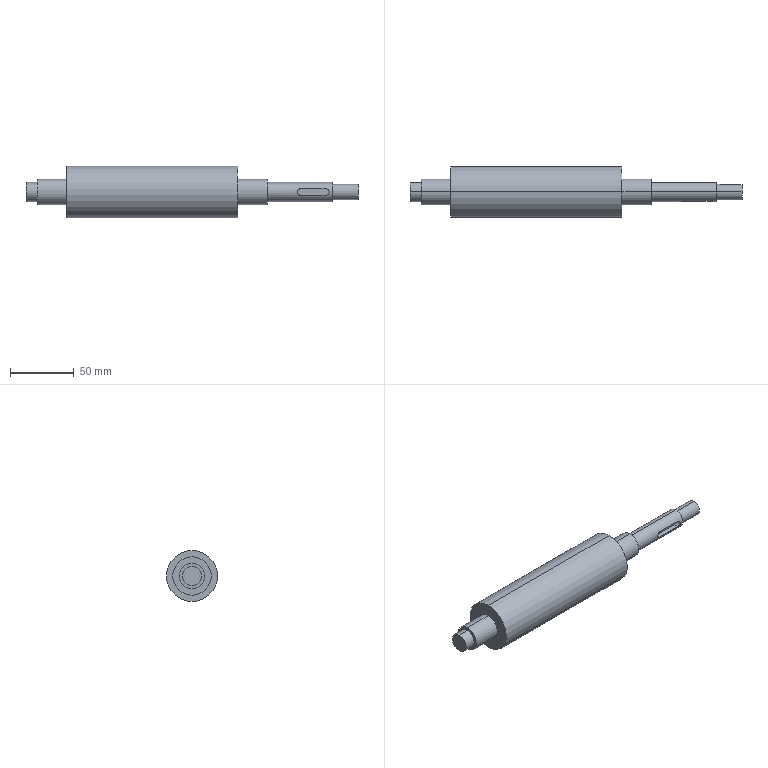Part | STEP file | MT-COMBO-119-S017 | 2 solids | 34 faces | box 260 x 40 x 40 mm | volume 195020 mm3 | cylinder 19 | plane 15 | commonest cylinder face diameters 15 x4 20 x4 30 x4 5 x2 12 x2 40 x2
STEP:
#1=CARTESIAN_POINT('',(-14.5,0.,-15.));
#2=VERTEX_POINT('',#1);
#3=CARTESIAN_POINT('',(-14.5,0.,15.));
#4=VERTEX_POINT('',#3);
#5=CARTESIAN_POINT('',(-14.5,0.,0.));
#6=DIRECTION('',(1.,0.,0.));
#7=DIRECTION('',(0.,0.,1.));
#8=AXIS2_PLACEMENT_3D('',#5,#6,#7);
#9=CIRCLE('',#8,15.);
#10=EDGE_CURVE('',#2,#4,#9,.T.);
#11=ORIENTED_EDGE('',*,*,#10,.F.);
#12=CARTESIAN_POINT('',(119.5,0.,-15.));
#13=VERTEX_POINT('',#12);
#14=CARTESIAN_POINT('',(-131.5,0.,-15.));
#15=DIRECTION('',(1.,0.,0.));
#16=VECTOR('',#15,1000.);
#17=LINE('',#14,#16);
#18=EDGE_CURVE('',#2,#13,#17,.T.);
#19=ORIENTED_EDGE('',*,*,#18,.T.);
#20=CARTESIAN_POINT('',(119.5,0.,15.));
#21=VERTEX_POINT('',#20);
#22=CARTESIAN_POINT('',(119.5,0.,0.));
#23=DIRECTION('',(-1.,0.,0.));
#24=DIRECTION('',(0.,0.,-1.));
#25=AXIS2_PLACEMENT_3D('',#22,#23,#24);
#26=CIRCLE('',#25,15.);
#27=EDGE_CURVE('',#21,#13,#26,.T.);
#28=ORIENTED_EDGE('',*,*,#27,.F.);
#29=CARTESIAN_POINT('',(-131.5,0.,15.));
#30=DIRECTION('',(1.,0.,0.));
#31=VECTOR('',#30,1000.);
#32=LINE('',#29,#31);
#33=EDGE_CURVE('',#4,#21,#32,.T.);
#34=ORIENTED_EDGE('',*,*,#33,.F.);
#35=EDGE_LOOP('',(#11,#19,#28,#34));
#36=FACE_OUTER_BOUND('',#35,.T.);
#37=CARTESIAN_POINT('',(-131.5,0.,0.));
#38=DIRECTION('',(1.,0.,0.));
#39=DIRECTION('',(0.,0.,1.));
#40=AXIS2_PLACEMENT_3D('',#37,#38,#39);
#41=CYLINDRICAL_SURFACE('',#40,15.);
#42=ADVANCED_FACE('',(#36),#41,.F.);
#43=CARTESIAN_POINT('',(-14.5,0.,-20.));
#44=VERTEX_POINT('',#43);
#45=CARTESIAN_POINT('',(-14.5,0.,20.));
#46=VERTEX_POINT('',#45);
#47=CARTESIAN_POINT('',(-14.5,0.,0.));
#48=DIRECTION('',(-1.,0.,0.));
#49=DIRECTION('',(0.,0.,1.));
#50=AXIS2_PLACEMENT_3D('',#47,#48,#49);
#51=CIRCLE('',#50,20.);
#52=EDGE_CURVE('',#44,#46,#51,.T.);
#53=ORIENTED_EDGE('',*,*,#52,.F.);
#54=CARTESIAN_POINT('',(119.5,0.,-20.));
#55=VERTEX_POINT('',#54);
#56=CARTESIAN_POINT('',(-131.5,0.,-20.));
#57=DIRECTION('',(1.,0.,0.));
#58=VECTOR('',#57,1000.);
#59=LINE('',#56,#58);
#60=EDGE_CURVE('',#44,#55,#59,.T.);
#61=ORIENTED_EDGE('',*,*,#60,.T.);
#62=CARTESIAN_POINT('',(119.5,0.,20.));
#63=VERTEX_POINT('',#62);
#64=CARTESIAN_POINT('',(119.5,0.,0.));
#65=DIRECTION('',(1.,0.,0.));
#66=DIRECTION('',(0.,0.,-1.));
#67=AXIS2_PLACEMENT_3D('',#64,#65,#66);
#68=CIRCLE('',#67,20.);
#69=EDGE_CURVE('',#63,#55,#68,.T.);
#70=ORIENTED_EDGE('',*,*,#69,.F.);
#71=CARTESIAN_POINT('',(-131.5,0.,20.));
#72=DIRECTION('',(1.,0.,0.));
#73=VECTOR('',#72,1000.);
#74=LINE('',#71,#73);
#75=EDGE_CURVE('',#46,#63,#74,.T.);
#76=ORIENTED_EDGE('',*,*,#75,.F.);
#77=EDGE_LOOP('',(#53,#61,#70,#76));
#78=FACE_OUTER_BOUND('',#77,.T.);
#79=CARTESIAN_POINT('',(-131.5,0.,0.));
#80=DIRECTION('',(1.,0.,0.));
#81=DIRECTION('',(0.,0.,1.));
#82=AXIS2_PLACEMENT_3D('',#79,#80,#81);
#83=CYLINDRICAL_SURFACE('',#82,20.);
#84=ADVANCED_FACE('',(#78),#83,.T.);
#85=ORIENTED_EDGE('',*,*,#60,.F.);
#86=CARTESIAN_POINT('',(-14.5,0.,0.));
#87=DIRECTION('',(-1.,0.,0.));
#88=DIRECTION('',(0.,0.,1.));
#89=AXIS2_PLACEMENT_3D('',#86,#87,#88);
#90=CIRCLE('',#89,20.);
#91=EDGE_CURVE('',#46,#44,#90,.T.);
#92=ORIENTED_EDGE('',*,*,#91,.F.);
#93=ORIENTED_EDGE('',*,*,#75,.T.);
#94=CARTESIAN_POINT('',(119.5,0.,0.));
#95=DIRECTION('',(1.,0.,0.));
#96=DIRECTION('',(0.,0.,-1.));
#97=AXIS2_PLACEMENT_3D('',#94,#95,#96);
#98=CIRCLE('',#97,20.);
#99=EDGE_CURVE('',#55,#63,#98,.T.);
#100=ORIENTED_EDGE('',*,*,#99,.F.);
#101=EDGE_LOOP('',(#85,#92,#93,#100));
#102=FACE_OUTER_BOUND('',#101,.T.);
#103=CARTESIAN_POINT('',(-131.5,0.,0.));
#104=DIRECTION('',(1.,0.,0.));
#105=DIRECTION('',(0.,0.,1.));
#106=AXIS2_PLACEMENT_3D('',#103,#104,#105);
#107=CYLINDRICAL_SURFACE('',#106,20.);
#108=ADVANCED_FACE('',(#102),#107,.T.);
#109=ORIENTED_EDGE('',*,*,#18,.F.);
#110=CARTESIAN_POINT('',(-14.5,0.,0.));
#111=DIRECTION('',(1.,0.,0.));
#112=DIRECTION('',(0.,0.,1.));
#113=AXIS2_PLACEMENT_3D('',#110,#111,#112);
#114=CIRCLE('',#113,15.);
#115=EDGE_CURVE('',#4,#2,#114,.T.);
#116=ORIENTED_EDGE('',*,*,#115,.F.);
#117=ORIENTED_EDGE('',*,*,#33,.T.);
#118=CARTESIAN_POINT('',(119.5,0.,0.));
#119=DIRECTION('',(-1.,0.,0.));
#120=DIRECTION('',(0.,0.,-1.));
#121=AXIS2_PLACEMENT_3D('',#118,#119,#120);
#122=CIRCLE('',#121,15.);
#123=EDGE_CURVE('',#13,#21,#122,.T.);
#124=ORIENTED_EDGE('',*,*,#123,.F.);
#125=EDGE_LOOP('',(#109,#116,#117,#124));
#126=FACE_OUTER_BOUND('',#125,.T.);
#127=CARTESIAN_POINT('',(-131.5,0.,0.));
#128=DIRECTION('',(1.,0.,0.));
#129=DIRECTION('',(0.,0.,1.));
#130=AXIS2_PLACEMENT_3D('',#127,#128,#129);
#131=CYLINDRICAL_SURFACE('',#130,15.);
#132=ADVANCED_FACE('',(#126),#131,.F.);
#133=ORIENTED_EDGE('',*,*,#91,.T.);
#134=ORIENTED_EDGE('',*,*,#52,.T.);
#135=EDGE_LOOP('',(#133,#134));
#136=FACE_OUTER_BOUND('',#135,.T.);
#137=ORIENTED_EDGE('',*,*,#115,.T.);
#138=ORIENTED_EDGE('',*,*,#10,.T.);
#139=EDGE_LOOP('',(#137,#138));
#140=FACE_BOUND('',#139,.T.);
#141=CARTESIAN_POINT('',(-14.5,0.,0.));
#142=DIRECTION('',(-1.,0.,0.));
#143=DIRECTION('',(0.,0.,1.));
#144=AXIS2_PLACEMENT_3D('',#141,#142,#143);
#145=PLANE('',#144);
#146=ADVANCED_FACE('',(#136,#140),#145,.T.);
#147=ORIENTED_EDGE('',*,*,#69,.T.);
#148=ORIENTED_EDGE('',*,*,#99,.T.);
#149=EDGE_LOOP('',(#147,#148));
#150=FACE_OUTER_BOUND('',#149,.T.);
#151=ORIENTED_EDGE('',*,*,#27,.T.);
#152=ORIENTED_EDGE('',*,*,#123,.T.);
#153=EDGE_LOOP('',(#151,#152));
#154=FACE_BOUND('',#153,.T.);
#155=CARTESIAN_POINT('',(119.5,0.,0.));
#156=DIRECTION('',(1.,0.,0.));
#157=DIRECTION('',(0.,0.,-1.));
#158=AXIS2_PLACEMENT_3D('',#155,#156,#157);
#159=PLANE('',#158);
#160=ADVANCED_FACE('',(#150,#154),#159,.T.);
#161=CLOSED_SHELL('',(#42,#84,#108,#132,#146,#160));
#162=MANIFOLD_SOLID_BREP('',#161);
#163=CARTESIAN_POINT('',(193.5,0.,-6.));
#164=VERTEX_POINT('',#163);
#165=CARTESIAN_POINT('',(193.5,0.,6.));
#166=VERTEX_POINT('',#165);
#167=CARTESIAN_POINT('',(193.5,0.,0.));
#168=DIRECTION('',(1.,0.,0.));
#169=DIRECTION('',(0.,0.,-1.));
#170=AXIS2_PLACEMENT_3D('',#167,#168,#169);
#171=CIRCLE('',#170,6.);
#172=EDGE_CURVE('',#164,#166,#171,.T.);
#173=ORIENTED_EDGE('',*,*,#172,.T.);
#174=CARTESIAN_POINT('',(213.5,0.,6.));
#175=VERTEX_POINT('',#174);
#176=CARTESIAN_POINT('',(193.5,0.,6.));
#177=DIRECTION('',(1.,0.,0.));
#178=VECTOR('',#177,1000.);
#179=LINE('',#176,#178);
#180=EDGE_CURVE('',#166,#175,#179,.T.);
#181=ORIENTED_EDGE('',*,*,#180,.T.);
#182=CARTESIAN_POINT('',(213.5,5.657,2.));
#183=VERTEX_POINT('',#182);
#184=CARTESIAN_POINT('',(213.5,0.,0.));
#185=DIRECTION('',(1.,0.,0.));
#186=DIRECTION('',(0.,0.,-1.));
#187=AXIS2_PLACEMENT_3D('',#184,#185,#186);
#188=CIRCLE('',#187,6.);
#189=EDGE_CURVE('',#183,#175,#188,.T.);
#190=ORIENTED_EDGE('',*,*,#189,.F.);
#191=CARTESIAN_POINT('',(198.,5.657,2.));
#192=VERTEX_POINT('',#191);
#193=CARTESIAN_POINT('',(193.5,5.657,2.));
#194=DIRECTION('',(1.,0.,0.));
#195=VECTOR('',#194,1000.);
#196=LINE('',#193,#195);
#197=EDGE_CURVE('',#192,#183,#196,.T.);
#198=ORIENTED_EDGE('',*,*,#197,.F.);
#199=CARTESIAN_POINT('',(198.,5.657,-2.));
#200=VERTEX_POINT('',#199);
#201=CARTESIAN_POINT('',(198.,5.657,-2.));
#202=CARTESIAN_POINT('',(197.867,5.657,-2.));
#203=CARTESIAN_POINT('',(197.736,5.662,-1.987));
#204=CARTESIAN_POINT('',(197.479,5.679,-1.935));
#205=CARTESIAN_POINT('',(197.352,5.693,-1.897));
#206=CARTESIAN_POINT('',(197.11,5.725,-1.796));
#207=CARTESIAN_POINT('',(196.996,5.744,-1.735));
#208=CARTESIAN_POINT('',(196.779,5.786,-1.59));
#209=CARTESIAN_POINT('',(196.677,5.809,-1.506));
#210=CARTESIAN_POINT('',(196.403,5.875,-1.231));
#211=CARTESIAN_POINT('',(196.254,5.919,-1.01));
#212=CARTESIAN_POINT('',(196.104,5.966,-0.6496));
#213=CARTESIAN_POINT('',(196.065,5.979,-0.5226));
#214=CARTESIAN_POINT('',(196.013,5.996,-0.264));
#215=CARTESIAN_POINT('',(196.,6.,-0.1336));
#216=CARTESIAN_POINT('',(196.,6.,0.1294));
#217=CARTESIAN_POINT('',(196.013,5.996,0.2629));
#218=CARTESIAN_POINT('',(196.064,5.979,0.5202));
#219=CARTESIAN_POINT('',(196.102,5.966,0.6454));
#220=CARTESIAN_POINT('',(196.204,5.935,0.8889));
#221=CARTESIAN_POINT('',(196.266,5.916,1.004));
#222=CARTESIAN_POINT('',(196.41,5.876,1.22));
#223=CARTESIAN_POINT('',(196.493,5.853,1.322));
#224=CARTESIAN_POINT('',(196.677,5.809,1.506));
#225=CARTESIAN_POINT('',(196.777,5.787,1.588));
#226=CARTESIAN_POINT('',(196.993,5.745,1.733));
#227=CARTESIAN_POINT('',(197.11,5.725,1.796));
#228=CARTESIAN_POINT('',(197.471,5.677,1.946));
#229=CARTESIAN_POINT('',(197.734,5.657,2.));
#230=CARTESIAN_POINT('',(198.,5.657,2.));
#231=B_SPLINE_CURVE_WITH_KNOTS('',3,(#201,#202,#203,#204,#205,#206,#207,#208,#209,#210,#211,#212,#213,#214,#215,#216,#217,#218,#219,#220,#221,#222,#223,#224,#225,#226,#227,#228,#229,#230),.UNSPECIFIED.,.F.,.F.,(4,2,2,2,2,2,2,2,2,2,2,2,2,2,4),(0.,0.0003935,0.000787,0.00118,0.001574,0.002361,0.002754,0.003148,0.003541,0.003935,0.004328,0.004722,0.005115,0.005509,0.006296),.UNSPECIFIED.);
#232=EDGE_CURVE('',#200,#192,#231,.T.);
#233=ORIENTED_EDGE('',*,*,#232,.F.);
#234=CARTESIAN_POINT('',(213.5,5.657,-2.));
#235=VERTEX_POINT('',#234);
#236=CARTESIAN_POINT('',(193.5,5.657,-2.));
#237=DIRECTION('',(-1.,0.,0.));
#238=VECTOR('',#237,1000.);
#239=LINE('',#236,#238);
#240=EDGE_CURVE('',#235,#200,#239,.T.);
#241=ORIENTED_EDGE('',*,*,#240,.F.);
#242=CARTESIAN_POINT('',(213.5,0.,-6.));
#243=VERTEX_POINT('',#242);
#244=CARTESIAN_POINT('',(213.5,0.,0.));
#245=DIRECTION('',(1.,0.,0.));
#246=DIRECTION('',(0.,0.,-1.));
#247=AXIS2_PLACEMENT_3D('',#244,#245,#246);
#248=CIRCLE('',#247,6.);
#249=EDGE_CURVE('',#243,#235,#248,.T.);
#250=ORIENTED_EDGE('',*,*,#249,.F.);
#251=CARTESIAN_POINT('',(193.5,0.,-6.));
#252=DIRECTION('',(1.,0.,0.));
#253=VECTOR('',#252,1000.);
#254=LINE('',#251,#253);
#255=EDGE_CURVE('',#164,#243,#254,.T.);
#256=ORIENTED_EDGE('',*,*,#255,.F.);
#257=EDGE_LOOP('',(#173,#181,#190,#198,#233,#241,#250,#256));
#258=FACE_OUTER_BOUND('',#257,.T.);
#259=CARTESIAN_POINT('',(193.5,0.,0.));
#260=DIRECTION('',(1.,0.,0.));
#261=DIRECTION('',(0.,0.,-1.));
#262=AXIS2_PLACEMENT_3D('',#259,#260,#261);
#263=CYLINDRICAL_SURFACE('',#262,6.);
#264=ADVANCED_FACE('',(#258),#263,.T.);
#265=CARTESIAN_POINT('',(119.5,0.,10.));
#266=VERTEX_POINT('',#265);
#267=CARTESIAN_POINT('',(119.5,0.,-10.));
#268=VERTEX_POINT('',#267);
#269=CARTESIAN_POINT('',(119.5,0.,0.));
#270=DIRECTION('',(1.,0.,0.));
#271=DIRECTION('',(0.,0.,-1.));
#272=AXIS2_PLACEMENT_3D('',#269,#270,#271);
#273=CIRCLE('',#272,10.);
#274=EDGE_CURVE('',#266,#268,#273,.T.);
#275=ORIENTED_EDGE('',*,*,#274,.T.);
#276=CARTESIAN_POINT('',(142.5,0.,-10.));
#277=VERTEX_POINT('',#276);
#278=CARTESIAN_POINT('',(0.,0.,-10.));
#279=DIRECTION('',(1.,0.,0.));
#280=VECTOR('',#279,1000.);
#281=LINE('',#278,#280);
#282=EDGE_CURVE('',#268,#277,#281,.T.);
#283=ORIENTED_EDGE('',*,*,#282,.T.);
#284=CARTESIAN_POINT('',(142.5,0.,10.));
#285=VERTEX_POINT('',#284);
#286=CARTESIAN_POINT('',(142.5,0.,0.));
#287=DIRECTION('',(-1.,0.,0.));
#288=DIRECTION('',(0.,0.,1.));
#289=AXIS2_PLACEMENT_3D('',#286,#287,#288);
#290=CIRCLE('',#289,10.);
#291=EDGE_CURVE('',#277,#285,#290,.T.);
#292=ORIENTED_EDGE('',*,*,#291,.T.);
#293=CARTESIAN_POINT('',(0.,0.,10.));
#294=DIRECTION('',(1.,0.,0.));
#295=VECTOR('',#294,1000.);
#296=LINE('',#293,#295);
#297=EDGE_CURVE('',#266,#285,#296,.T.);
#298=ORIENTED_EDGE('',*,*,#297,.F.);
#299=EDGE_LOOP('',(#275,#283,#292,#298));
#300=FACE_OUTER_BOUND('',#299,.T.);
#301=CARTESIAN_POINT('',(0.,0.,0.));
#302=DIRECTION('',(1.,0.,0.));
#303=DIRECTION('',(0.,0.,1.));
#304=AXIS2_PLACEMENT_3D('',#301,#302,#303);
#305=CYLINDRICAL_SURFACE('',#304,10.);
#306=ADVANCED_FACE('',(#300),#305,.T.);
#307=CARTESIAN_POINT('',(-37.5,0.,-10.));
#308=VERTEX_POINT('',#307);
#309=CARTESIAN_POINT('',(-37.5,0.,10.));
#310=VERTEX_POINT('',#309);
#311=CARTESIAN_POINT('',(-37.5,0.,0.));
#312=DIRECTION('',(-1.,0.,0.));
#313=DIRECTION('',(0.,0.,1.));
#314=AXIS2_PLACEMENT_3D('',#311,#312,#313);
#315=CIRCLE('',#314,10.);
#316=EDGE_CURVE('',#308,#310,#315,.T.);
#317=ORIENTED_EDGE('',*,*,#316,.F.);
#318=CARTESIAN_POINT('',(-14.5,0.,-10.));
#319=VERTEX_POINT('',#318);
#320=CARTESIAN_POINT('',(0.,0.,-10.));
#321=DIRECTION('',(1.,0.,0.));
#322=VECTOR('',#321,1000.);
#323=LINE('',#320,#322);
#324=EDGE_CURVE('',#308,#319,#323,.T.);
#325=ORIENTED_EDGE('',*,*,#324,.T.);
#326=CARTESIAN_POINT('',(-14.5,0.,10.));
#327=VERTEX_POINT('',#326);
#328=CARTESIAN_POINT('',(-14.5,0.,0.));
#329=DIRECTION('',(-1.,0.,0.));
#330=DIRECTION('',(0.,0.,1.));
#331=AXIS2_PLACEMENT_3D('',#328,#329,#330);
#332=CIRCLE('',#331,10.);
#333=EDGE_CURVE('',#319,#327,#332,.T.);
#334=ORIENTED_EDGE('',*,*,#333,.T.);
#335=CARTESIAN_POINT('',(0.,0.,10.));
#336=DIRECTION('',(1.,0.,0.));
#337=VECTOR('',#336,1000.);
#338=LINE('',#335,#337);
#339=EDGE_CURVE('',#310,#327,#338,.T.);
#340=ORIENTED_EDGE('',*,*,#339,.F.);
#341=EDGE_LOOP('',(#317,#325,#334,#340));
#342=FACE_OUTER_BOUND('',#341,.T.);
#343=CARTESIAN_POINT('',(0.,0.,0.));
#344=DIRECTION('',(1.,0.,0.));
#345=DIRECTION('',(0.,0.,1.));
#346=AXIS2_PLACEMENT_3D('',#343,#344,#345);
#347=CYLINDRICAL_SURFACE('',#346,10.);
#348=ADVANCED_FACE('',(#342),#347,.T.);
#349=CARTESIAN_POINT('',(-46.5,0.,-7.5));
#350=VERTEX_POINT('',#349);
#351=CARTESIAN_POINT('',(-46.5,0.,7.5));
#352=VERTEX_POINT('',#351);
#353=CARTESIAN_POINT('',(-46.5,0.,0.));
#354=DIRECTION('',(-1.,0.,0.));
#355=DIRECTION('',(0.,0.,1.));
#356=AXIS2_PLACEMENT_3D('',#353,#354,#355);
#357=CIRCLE('',#356,7.5);
#358=EDGE_CURVE('',#350,#352,#357,.T.);
#359=ORIENTED_EDGE('',*,*,#358,.F.);
#360=CARTESIAN_POINT('',(-37.5,0.,-7.5));
#361=VERTEX_POINT('',#360);
#362=CARTESIAN_POINT('',(0.,0.,-7.5));
#363=DIRECTION('',(1.,0.,0.));
#364=VECTOR('',#363,1000.);
#365=LINE('',#362,#364);
#366=EDGE_CURVE('',#350,#361,#365,.T.);
#367=ORIENTED_EDGE('',*,*,#366,.T.);
#368=CARTESIAN_POINT('',(-37.5,0.,7.5));
#369=VERTEX_POINT('',#368);
#370=CARTESIAN_POINT('',(-37.5,0.,0.));
#371=DIRECTION('',(-1.,0.,0.));
#372=DIRECTION('',(0.,0.,1.));
#373=AXIS2_PLACEMENT_3D('',#370,#371,#372);
#374=CIRCLE('',#373,7.5);
#375=EDGE_CURVE('',#361,#369,#374,.T.);
#376=ORIENTED_EDGE('',*,*,#375,.T.);
#377=CARTESIAN_POINT('',(0.,0.,7.5));
#378=DIRECTION('',(1.,0.,0.));
#379=VECTOR('',#378,1000.);
#380=LINE('',#377,#379);
#381=EDGE_CURVE('',#352,#369,#380,.T.);
#382=ORIENTED_EDGE('',*,*,#381,.F.);
#383=EDGE_LOOP('',(#359,#367,#376,#382));
#384=FACE_OUTER_BOUND('',#383,.T.);
#385=CARTESIAN_POINT('',(0.,0.,0.));
#386=DIRECTION('',(1.,0.,0.));
#387=DIRECTION('',(0.,0.,1.));
#388=AXIS2_PLACEMENT_3D('',#385,#386,#387);
#389=CYLINDRICAL_SURFACE('',#388,7.5);
#390=ADVANCED_FACE('',(#384),#389,.T.);
#391=CARTESIAN_POINT('',(-14.5,0.,15.));
#392=VERTEX_POINT('',#391);
#393=CARTESIAN_POINT('',(-14.5,0.,-15.));
#394=VERTEX_POINT('',#393);
#395=CARTESIAN_POINT('',(-14.5,0.,0.));
#396=DIRECTION('',(1.,0.,0.));
#397=DIRECTION('',(0.,0.,1.));
#398=AXIS2_PLACEMENT_3D('',#395,#396,#397);
#399=CIRCLE('',#398,15.);
#400=EDGE_CURVE('',#392,#394,#399,.T.);
#401=ORIENTED_EDGE('',*,*,#400,.T.);
#402=CARTESIAN_POINT('',(119.5,0.,-15.));
#403=VERTEX_POINT('',#402);
#404=CARTESIAN_POINT('',(0.,0.,-15.));
#405=DIRECTION('',(1.,0.,0.));
#406=VECTOR('',#405,1000.);
#407=LINE('',#404,#406);
#408=EDGE_CURVE('',#394,#403,#407,.T.);
#409=ORIENTED_EDGE('',*,*,#408,.T.);
#410=CARTESIAN_POINT('',(119.5,0.,15.));
#411=VERTEX_POINT('',#410);
#412=CARTESIAN_POINT('',(119.5,0.,0.));
#413=DIRECTION('',(-1.,0.,0.));
#414=DIRECTION('',(0.,0.,-1.));
#415=AXIS2_PLACEMENT_3D('',#412,#413,#414);
#416=CIRCLE('',#415,15.);
#417=EDGE_CURVE('',#403,#411,#416,.T.);
#418=ORIENTED_EDGE('',*,*,#417,.T.);
#419=CARTESIAN_POINT('',(0.,0.,15.));
#420=DIRECTION('',(1.,0.,0.));
#421=VECTOR('',#420,1000.);
#422=LINE('',#419,#421);
#423=EDGE_CURVE('',#392,#411,#422,.T.);
#424=ORIENTED_EDGE('',*,*,#423,.F.);
#425=EDGE_LOOP('',(#401,#409,#418,#424));
#426=FACE_OUTER_BOUND('',#425,.T.);
#427=CARTESIAN_POINT('',(0.,0.,0.));
#428=DIRECTION('',(1.,0.,0.));
#429=DIRECTION('',(0.,0.,1.));
#430=AXIS2_PLACEMENT_3D('',#427,#428,#429);
#431=CYLINDRICAL_SURFACE('',#430,15.);
#432=ADVANCED_FACE('',(#426),#431,.T.);
#433=CARTESIAN_POINT('',(188.5,-7.071,-2.5));
#434=VERTEX_POINT('',#433);
#435=CARTESIAN_POINT('',(188.5,-7.071,2.5));
#436=VERTEX_POINT('',#435);
#437=CARTESIAN_POINT('',(188.5,-7.071,-2.5));
#438=CARTESIAN_POINT('',(188.666,-7.071,-2.5));
#439=CARTESIAN_POINT('',(188.83,-7.077,-2.484));
#440=CARTESIAN_POINT('',(189.151,-7.099,-2.419));
#441=CARTESIAN_POINT('',(189.31,-7.116,-2.371));
#442=CARTESIAN_POINT('',(189.612,-7.156,-2.245));
#443=CARTESIAN_POINT('',(189.755,-7.18,-2.168));
#444=CARTESIAN_POINT('',(190.026,-7.233,-1.987));
#445=CARTESIAN_POINT('',(190.153,-7.261,-1.882));
#446=CARTESIAN_POINT('',(190.496,-7.344,-1.539));
#447=CARTESIAN_POINT('',(190.682,-7.399,-1.262));
#448=CARTESIAN_POINT('',(190.87,-7.457,-0.812));
#449=CARTESIAN_POINT('',(190.919,-7.473,-0.6532));
#450=CARTESIAN_POINT('',(190.984,-7.494,-0.33));
#451=CARTESIAN_POINT('',(191.,-7.5,-0.167));
#452=CARTESIAN_POINT('',(191.,-7.5,0.1617));
#453=CARTESIAN_POINT('',(190.984,-7.495,0.3287));
#454=CARTESIAN_POINT('',(190.92,-7.473,0.6503));
#455=CARTESIAN_POINT('',(190.872,-7.458,0.8068));
#456=CARTESIAN_POINT('',(190.746,-7.419,1.111));
#457=CARTESIAN_POINT('',(190.668,-7.395,1.255));
#458=CARTESIAN_POINT('',(190.488,-7.345,1.525));
#459=CARTESIAN_POINT('',(190.383,-7.317,1.652));
#460=CARTESIAN_POINT('',(190.153,-7.261,1.882));
#461=CARTESIAN_POINT('',(190.028,-7.233,1.985));
#462=CARTESIAN_POINT('',(189.759,-7.181,2.166));
#463=CARTESIAN_POINT('',(189.613,-7.156,2.245));
#464=CARTESIAN_POINT('',(189.312,-7.116,2.37));
#465=CARTESIAN_POINT('',(189.156,-7.1,2.418));
#466=CARTESIAN_POINT('',(188.833,-7.077,2.483));
#467=CARTESIAN_POINT('',(188.666,-7.071,2.5));
#468=CARTESIAN_POINT('',(188.5,-7.071,2.5));
#469=B_SPLINE_CURVE_WITH_KNOTS('',3,(#437,#438,#439,#440,#441,#442,#443,#444,#445,#446,#447,#448,#449,#450,#451,#452,#453,#454,#455,#456,#457,#458,#459,#460,#461,#462,#463,#464,#465,#466,#467,#468),.UNSPECIFIED.,.F.,.F.,(4,2,2,2,2,2,2,2,2,2,2,2,2,2,2,4),(0.,0.0004919,0.0009837,0.001476,0.001967,0.002951,0.003443,0.003935,0.004427,0.004919,0.00541,0.005902,0.006394,0.006886,0.007378,0.00787),.UNSPECIFIED.);
#470=EDGE_CURVE('',#434,#436,#469,.T.);
#471=ORIENTED_EDGE('',*,*,#470,.F.);
#472=CARTESIAN_POINT('',(168.5,-7.071,-2.5));
#473=VERTEX_POINT('',#472);
#474=CARTESIAN_POINT('',(0.,-7.071,-2.5));
#475=DIRECTION('',(1.,0.,0.));
#476=VECTOR('',#475,1000.);
#477=LINE('',#474,#476);
#478=EDGE_CURVE('',#473,#434,#477,.T.);
#479=ORIENTED_EDGE('',*,*,#478,.F.);
#480=CARTESIAN_POINT('',(168.5,-7.071,2.5));
#481=VERTEX_POINT('',#480);
#482=CARTESIAN_POINT('',(168.5,-7.071,2.5));
#483=CARTESIAN_POINT('',(168.334,-7.071,2.5));
#484=CARTESIAN_POINT('',(168.17,-7.077,2.484));
#485=CARTESIAN_POINT('',(167.849,-7.099,2.419));
#486=CARTESIAN_POINT('',(167.69,-7.116,2.371));
#487=CARTESIAN_POINT('',(167.388,-7.156,2.245));
#488=CARTESIAN_POINT('',(167.245,-7.18,2.168));
#489=CARTESIAN_POINT('',(166.974,-7.233,1.987));
#490=CARTESIAN_POINT('',(166.847,-7.261,1.882));
#491=CARTESIAN_POINT('',(166.504,-7.344,1.539));
#492=CARTESIAN_POINT('',(166.318,-7.399,1.262));
#493=CARTESIAN_POINT('',(166.13,-7.457,0.812));
#494=CARTESIAN_POINT('',(166.081,-7.473,0.6532));
#495=CARTESIAN_POINT('',(166.016,-7.494,0.33));
#496=CARTESIAN_POINT('',(166.,-7.5,0.167));
#497=CARTESIAN_POINT('',(166.,-7.5,-0.1617));
#498=CARTESIAN_POINT('',(166.016,-7.495,-0.3287));
#499=CARTESIAN_POINT('',(166.08,-7.473,-0.6503));
#500=CARTESIAN_POINT('',(166.128,-7.458,-0.8068));
#501=CARTESIAN_POINT('',(166.254,-7.419,-1.111));
#502=CARTESIAN_POINT('',(166.332,-7.395,-1.255));
#503=CARTESIAN_POINT('',(166.512,-7.345,-1.525));
#504=CARTESIAN_POINT('',(166.617,-7.317,-1.652));
#505=CARTESIAN_POINT('',(166.847,-7.261,-1.882));
#506=CARTESIAN_POINT('',(166.972,-7.233,-1.985));
#507=CARTESIAN_POINT('',(167.241,-7.181,-2.166));
#508=CARTESIAN_POINT('',(167.387,-7.156,-2.245));
#509=CARTESIAN_POINT('',(167.688,-7.116,-2.37));
#510=CARTESIAN_POINT('',(167.844,-7.1,-2.418));
#511=CARTESIAN_POINT('',(168.167,-7.077,-2.483));
#512=CARTESIAN_POINT('',(168.334,-7.071,-2.5));
#513=CARTESIAN_POINT('',(168.5,-7.071,-2.5));
#514=B_SPLINE_CURVE_WITH_KNOTS('',3,(#482,#483,#484,#485,#486,#487,#488,#489,#490,#491,#492,#493,#494,#495,#496,#497,#498,#499,#500,#501,#502,#503,#504,#505,#506,#507,#508,#509,#510,#511,#512,#513),.UNSPECIFIED.,.F.,.F.,(4,2,2,2,2,2,2,2,2,2,2,2,2,2,2,4),(0.,0.0004919,0.0009837,0.001476,0.001967,0.002951,0.003443,0.003935,0.004427,0.004919,0.00541,0.005902,0.006394,0.006886,0.007378,0.00787),.UNSPECIFIED.);
#515=EDGE_CURVE('',#481,#473,#514,.T.);
#516=ORIENTED_EDGE('',*,*,#515,.F.);
#517=CARTESIAN_POINT('',(0.,-7.071,2.5));
#518=DIRECTION('',(-1.,0.,0.));
#519=VECTOR('',#518,1000.);
#520=LINE('',#517,#519);
#521=EDGE_CURVE('',#436,#481,#520,.T.);
#522=ORIENTED_EDGE('',*,*,#521,.F.);
#523=EDGE_LOOP('',(#471,#479,#516,#522));
#524=FACE_BOUND('',#523,.T.);
#525=CARTESIAN_POINT('',(142.5,0.,-7.5));
#526=VERTEX_POINT('',#525);
#527=CARTESIAN_POINT('',(142.5,0.,7.5));
#528=VERTEX_POINT('',#527);
#529=CARTESIAN_POINT('',(142.5,0.,0.));
#530=DIRECTION('',(-1.,0.,0.));
#531=DIRECTION('',(0.,0.,1.));
#532=AXIS2_PLACEMENT_3D('',#529,#530,#531);
#533=CIRCLE('',#532,7.5);
#534=EDGE_CURVE('',#526,#528,#533,.T.);
#535=ORIENTED_EDGE('',*,*,#534,.F.);
#536=CARTESIAN_POINT('',(193.5,0.,-7.5));
#537=VERTEX_POINT('',#536);
#538=CARTESIAN_POINT('',(0.,0.,-7.5));
#539=DIRECTION('',(1.,0.,0.));
#540=VECTOR('',#539,1000.);
#541=LINE('',#538,#540);
#542=EDGE_CURVE('',#526,#537,#541,.T.);
#543=ORIENTED_EDGE('',*,*,#542,.T.);
#544=CARTESIAN_POINT('',(193.5,0.,7.5));
#545=VERTEX_POINT('',#544);
#546=CARTESIAN_POINT('',(193.5,0.,0.));
#547=DIRECTION('',(1.,0.,0.));
#548=DIRECTION('',(0.,0.,-1.));
#549=AXIS2_PLACEMENT_3D('',#546,#547,#548);
#550=CIRCLE('',#549,7.5);
#551=EDGE_CURVE('',#545,#537,#550,.T.);
#552=ORIENTED_EDGE('',*,*,#551,.F.);
#553=CARTESIAN_POINT('',(0.,0.,7.5));
#554=DIRECTION('',(1.,0.,0.));
#555=VECTOR('',#554,1000.);
#556=LINE('',#553,#555);
#557=EDGE_CURVE('',#528,#545,#556,.T.);
#558=ORIENTED_EDGE('',*,*,#557,.F.);
#559=EDGE_LOOP('',(#535,#543,#552,#558));
#560=FACE_OUTER_BOUND('',#559,.T.);
#561=CARTESIAN_POINT('',(0.,0.,0.));
#562=DIRECTION('',(1.,0.,0.));
#563=DIRECTION('',(0.,0.,1.));
#564=AXIS2_PLACEMENT_3D('',#561,#562,#563);
#565=CYLINDRICAL_SURFACE('',#564,7.5);
#566=ADVANCED_FACE('',(#524,#560),#565,.T.);
#567=ORIENTED_EDGE('',*,*,#542,.F.);
#568=CARTESIAN_POINT('',(142.5,0.,0.));
#569=DIRECTION('',(-1.,0.,0.));
#570=DIRECTION('',(0.,0.,1.));
#571=AXIS2_PLACEMENT_3D('',#568,#569,#570);
#572=CIRCLE('',#571,7.5);
#573=EDGE_CURVE('',#528,#526,#572,.T.);
#574=ORIENTED_EDGE('',*,*,#573,.F.);
#575=ORIENTED_EDGE('',*,*,#557,.T.);
#576=CARTESIAN_POINT('',(193.5,0.,0.));
#577=DIRECTION('',(1.,0.,0.));
#578=DIRECTION('',(0.,0.,-1.));
#579=AXIS2_PLACEMENT_3D('',#576,#577,#578);
#580=CIRCLE('',#579,7.5);
#581=EDGE_CURVE('',#537,#545,#580,.T.);
#582=ORIENTED_EDGE('',*,*,#581,.F.);
#583=EDGE_LOOP('',(#567,#574,#575,#582));
#584=FACE_OUTER_BOUND('',#583,.T.);
#585=CARTESIAN_POINT('',(0.,0.,0.));
#586=DIRECTION('',(1.,0.,0.));
#587=DIRECTION('',(0.,0.,1.));
#588=AXIS2_PLACEMENT_3D('',#585,#586,#587);
#589=CYLINDRICAL_SURFACE('',#588,7.5);
#590=ADVANCED_FACE('',(#584),#589,.T.);
#591=ORIENTED_EDGE('',*,*,#408,.F.);
#592=CARTESIAN_POINT('',(-14.5,0.,0.));
#593=DIRECTION('',(1.,0.,0.));
#594=DIRECTION('',(0.,0.,1.));
#595=AXIS2_PLACEMENT_3D('',#592,#593,#594);
#596=CIRCLE('',#595,15.);
#597=EDGE_CURVE('',#394,#392,#596,.T.);
#598=ORIENTED_EDGE('',*,*,#597,.T.);
#599=ORIENTED_EDGE('',*,*,#423,.T.);
#600=CARTESIAN_POINT('',(119.5,0.,0.));
#601=DIRECTION('',(-1.,0.,0.));
#602=DIRECTION('',(0.,0.,-1.));
#603=AXIS2_PLACEMENT_3D('',#600,#601,#602);
#604=CIRCLE('',#603,15.);
#605=EDGE_CURVE('',#411,#403,#604,.T.);
#606=ORIENTED_EDGE('',*,*,#605,.T.);
#607=EDGE_LOOP('',(#591,#598,#599,#606));
#608=FACE_OUTER_BOUND('',#607,.T.);
#609=CARTESIAN_POINT('',(0.,0.,0.));
#610=DIRECTION('',(1.,0.,0.));
#611=DIRECTION('',(0.,0.,1.));
#612=AXIS2_PLACEMENT_3D('',#609,#610,#611);
#613=CYLINDRICAL_SURFACE('',#612,15.);
#614=ADVANCED_FACE('',(#608),#613,.T.);
#615=ORIENTED_EDGE('',*,*,#400,.F.);
#616=ORIENTED_EDGE('',*,*,#597,.F.);
#617=EDGE_LOOP('',(#615,#616));
#618=FACE_OUTER_BOUND('',#617,.T.);
#619=CARTESIAN_POINT('',(-14.5,0.,0.));
#620=DIRECTION('',(-1.,0.,0.));
#621=DIRECTION('',(0.,0.,1.));
#622=AXIS2_PLACEMENT_3D('',#619,#620,#621);
#623=CIRCLE('',#622,10.);
#624=EDGE_CURVE('',#327,#319,#623,.T.);
#625=ORIENTED_EDGE('',*,*,#624,.F.);
#626=ORIENTED_EDGE('',*,*,#333,.F.);
#627=EDGE_LOOP('',(#625,#626));
#628=FACE_BOUND('',#627,.T.);
#629=CARTESIAN_POINT('',(-14.5,0.,0.));
#630=DIRECTION('',(-1.,0.,0.));
#631=DIRECTION('',(0.,0.,1.));
#632=AXIS2_PLACEMENT_3D('',#629,#630,#631);
#633=PLANE('',#632);
#634=ADVANCED_FACE('',(#618,#628),#633,.T.);
#635=CARTESIAN_POINT('',(-46.5,0.,0.));
#636=DIRECTION('',(-1.,0.,0.));
#637=DIRECTION('',(0.,0.,1.));
#638=AXIS2_PLACEMENT_3D('',#635,#636,#637);
#639=CIRCLE('',#638,7.5);
#640=EDGE_CURVE('',#352,#350,#639,.T.);
#641=ORIENTED_EDGE('',*,*,#640,.T.);
#642=ORIENTED_EDGE('',*,*,#358,.T.);
#643=EDGE_LOOP('',(#641,#642));
#644=FACE_OUTER_BOUND('',#643,.T.);
#645=CARTESIAN_POINT('',(-46.5,0.,0.));
#646=DIRECTION('',(-1.,0.,0.));
#647=DIRECTION('',(0.,0.,-1.));
#648=AXIS2_PLACEMENT_3D('',#645,#646,#647);
#649=PLANE('',#648);
#650=ADVANCED_FACE('',(#644),#649,.T.);
#651=ORIENTED_EDGE('',*,*,#366,.F.);
#652=ORIENTED_EDGE('',*,*,#640,.F.);
#653=ORIENTED_EDGE('',*,*,#381,.T.);
#654=CARTESIAN_POINT('',(-37.5,0.,0.));
#655=DIRECTION('',(-1.,0.,0.));
#656=DIRECTION('',(0.,0.,1.));
#657=AXIS2_PLACEMENT_3D('',#654,#655,#656);
#658=CIRCLE('',#657,7.5);
#659=EDGE_CURVE('',#369,#361,#658,.T.);
#660=ORIENTED_EDGE('',*,*,#659,.T.);
#661=EDGE_LOOP('',(#651,#652,#653,#660));
#662=FACE_OUTER_BOUND('',#661,.T.);
#663=CARTESIAN_POINT('',(0.,0.,0.));
#664=DIRECTION('',(1.,0.,0.));
#665=DIRECTION('',(0.,0.,1.));
#666=AXIS2_PLACEMENT_3D('',#663,#664,#665);
#667=CYLINDRICAL_SURFACE('',#666,7.5);
#668=ADVANCED_FACE('',(#662),#667,.T.);
#669=ORIENTED_EDGE('',*,*,#659,.F.);
#670=ORIENTED_EDGE('',*,*,#375,.F.);
#671=EDGE_LOOP('',(#669,#670));
#672=FACE_BOUND('',#671,.T.);
#673=CARTESIAN_POINT('',(-37.5,0.,0.));
#674=DIRECTION('',(-1.,0.,0.));
#675=DIRECTION('',(0.,0.,1.));
#676=AXIS2_PLACEMENT_3D('',#673,#674,#675);
#677=CIRCLE('',#676,10.);
#678=EDGE_CURVE('',#310,#308,#677,.T.);
#679=ORIENTED_EDGE('',*,*,#678,.T.);
#680=ORIENTED_EDGE('',*,*,#316,.T.);
#681=EDGE_LOOP('',(#679,#680));
#682=FACE_OUTER_BOUND('',#681,.T.);
#683=CARTESIAN_POINT('',(-37.5,7.5,0.));
#684=DIRECTION('',(-1.,0.,0.));
#685=DIRECTION('',(0.,0.,-1.));
#686=AXIS2_PLACEMENT_3D('',#683,#684,#685);
#687=PLANE('',#686);
#688=ADVANCED_FACE('',(#672,#682),#687,.T.);
#689=ORIENTED_EDGE('',*,*,#324,.F.);
#690=ORIENTED_EDGE('',*,*,#678,.F.);
#691=ORIENTED_EDGE('',*,*,#339,.T.);
#692=ORIENTED_EDGE('',*,*,#624,.T.);
#693=EDGE_LOOP('',(#689,#690,#691,#692));
#694=FACE_OUTER_BOUND('',#693,.T.);
#695=CARTESIAN_POINT('',(0.,0.,0.));
#696=DIRECTION('',(1.,0.,0.));
#697=DIRECTION('',(0.,0.,1.));
#698=AXIS2_PLACEMENT_3D('',#695,#696,#697);
#699=CYLINDRICAL_SURFACE('',#698,10.);
#700=ADVANCED_FACE('',(#694),#699,.T.);
#701=ORIENTED_EDGE('',*,*,#605,.F.);
#702=ORIENTED_EDGE('',*,*,#417,.F.);
#703=EDGE_LOOP('',(#701,#702));
#704=FACE_OUTER_BOUND('',#703,.T.);
#705=ORIENTED_EDGE('',*,*,#274,.F.);
#706=CARTESIAN_POINT('',(119.5,0.,0.));
#707=DIRECTION('',(1.,0.,0.));
#708=DIRECTION('',(0.,0.,-1.));
#709=AXIS2_PLACEMENT_3D('',#706,#707,#708);
#710=CIRCLE('',#709,10.);
#711=EDGE_CURVE('',#268,#266,#710,.T.);
#712=ORIENTED_EDGE('',*,*,#711,.F.);
#713=EDGE_LOOP('',(#705,#712));
#714=FACE_BOUND('',#713,.T.);
#715=CARTESIAN_POINT('',(119.5,0.,0.));
#716=DIRECTION('',(1.,0.,0.));
#717=DIRECTION('',(0.,0.,-1.));
#718=AXIS2_PLACEMENT_3D('',#715,#716,#717);
#719=PLANE('',#718);
#720=ADVANCED_FACE('',(#704,#714),#719,.T.);
#721=CARTESIAN_POINT('',(168.5,-3.,2.5));
#722=VERTEX_POINT('',#721);
#723=CARTESIAN_POINT('',(168.5,-3.,-2.5));
#724=VERTEX_POINT('',#723);
#725=CARTESIAN_POINT('',(168.5,-3.,0.));
#726=DIRECTION('',(0.,-1.,0.));
#727=DIRECTION('',(0.,0.,-1.));
#728=AXIS2_PLACEMENT_3D('',#725,#726,#727);
#729=CIRCLE('',#728,2.5);
#730=EDGE_CURVE('',#722,#724,#729,.T.);
#731=ORIENTED_EDGE('',*,*,#730,.T.);
#732=CARTESIAN_POINT('',(188.5,-3.,-2.5));
#733=VERTEX_POINT('',#732);
#734=CARTESIAN_POINT('',(168.5,-3.,-2.5));
#735=DIRECTION('',(1.,0.,0.));
#736=VECTOR('',#735,1000.);
#737=LINE('',#734,#736);
#738=EDGE_CURVE('',#724,#733,#737,.T.);
#739=ORIENTED_EDGE('',*,*,#738,.T.);
#740=CARTESIAN_POINT('',(188.5,-3.,2.5));
#741=VERTEX_POINT('',#740);
#742=CARTESIAN_POINT('',(188.5,-3.,0.));
#743=DIRECTION('',(0.,-1.,0.));
#744=DIRECTION('',(0.,0.,-1.));
#745=AXIS2_PLACEMENT_3D('',#742,#743,#744);
#746=CIRCLE('',#745,2.5);
#747=EDGE_CURVE('',#733,#741,#746,.T.);
#748=ORIENTED_EDGE('',*,*,#747,.T.);
#749=CARTESIAN_POINT('',(168.5,-3.,2.5));
#750=DIRECTION('',(-1.,0.,0.));
#751=VECTOR('',#750,1000.);
#752=LINE('',#749,#751);
#753=EDGE_CURVE('',#741,#722,#752,.T.);
#754=ORIENTED_EDGE('',*,*,#753,.T.);
#755=EDGE_LOOP('',(#731,#739,#748,#754));
#756=FACE_OUTER_BOUND('',#755,.T.);
#757=CARTESIAN_POINT('',(168.5,-3.,0.));
#758=DIRECTION('',(0.,-1.,0.));
#759=DIRECTION('',(0.,0.,-1.));
#760=AXIS2_PLACEMENT_3D('',#757,#758,#759);
#761=PLANE('',#760);
#762=ADVANCED_FACE('',(#756),#761,.T.);
#763=ORIENTED_EDGE('',*,*,#521,.T.);
#764=CARTESIAN_POINT('',(168.5,-3.,2.5));
#765=DIRECTION('',(0.,-1.,0.));
#766=VECTOR('',#765,1000.);
#767=LINE('',#764,#766);
#768=EDGE_CURVE('',#722,#481,#767,.T.);
#769=ORIENTED_EDGE('',*,*,#768,.F.);
#770=ORIENTED_EDGE('',*,*,#753,.F.);
#771=CARTESIAN_POINT('',(188.5,-3.,2.5));
#772=DIRECTION('',(0.,-1.,0.));
#773=VECTOR('',#772,1000.);
#774=LINE('',#771,#773);
#775=EDGE_CURVE('',#741,#436,#774,.T.);
#776=ORIENTED_EDGE('',*,*,#775,.T.);
#777=EDGE_LOOP('',(#763,#769,#770,#776));
#778=FACE_OUTER_BOUND('',#777,.T.);
#779=CARTESIAN_POINT('',(168.5,-3.,2.5));
#780=DIRECTION('',(0.,0.,1.));
#781=DIRECTION('',(1.,0.,0.));
#782=AXIS2_PLACEMENT_3D('',#779,#780,#781);
#783=PLANE('',#782);
#784=ADVANCED_FACE('',(#778),#783,.F.);
#785=ORIENTED_EDGE('',*,*,#768,.T.);
#786=ORIENTED_EDGE('',*,*,#515,.T.);
#787=CARTESIAN_POINT('',(168.5,-3.,-2.5));
#788=DIRECTION('',(0.,-1.,0.));
#789=VECTOR('',#788,1000.);
#790=LINE('',#787,#789);
#791=EDGE_CURVE('',#724,#473,#790,.T.);
#792=ORIENTED_EDGE('',*,*,#791,.F.);
#793=ORIENTED_EDGE('',*,*,#730,.F.);
#794=EDGE_LOOP('',(#785,#786,#792,#793));
#795=FACE_OUTER_BOUND('',#794,.T.);
#796=CARTESIAN_POINT('',(168.5,-3.,0.));
#797=DIRECTION('',(0.,-1.,0.));
#798=DIRECTION('',(0.,0.,-1.));
#799=AXIS2_PLACEMENT_3D('',#796,#797,#798);
#800=CYLINDRICAL_SURFACE('',#799,2.5);
#801=ADVANCED_FACE('',(#795),#800,.F.);
#802=ORIENTED_EDGE('',*,*,#478,.T.);
#803=CARTESIAN_POINT('',(188.5,-3.,-2.5));
#804=DIRECTION('',(0.,-1.,0.));
#805=VECTOR('',#804,1000.);
#806=LINE('',#803,#805);
#807=EDGE_CURVE('',#733,#434,#806,.T.);
#808=ORIENTED_EDGE('',*,*,#807,.F.);
#809=ORIENTED_EDGE('',*,*,#738,.F.);
#810=ORIENTED_EDGE('',*,*,#791,.T.);
#811=EDGE_LOOP('',(#802,#808,#809,#810));
#812=FACE_OUTER_BOUND('',#811,.T.);
#813=CARTESIAN_POINT('',(168.5,-3.,-2.5));
#814=DIRECTION('',(0.,0.,-1.));
#815=DIRECTION('',(-1.,0.,0.));
#816=AXIS2_PLACEMENT_3D('',#813,#814,#815);
#817=PLANE('',#816);
#818=ADVANCED_FACE('',(#812),#817,.F.);
#819=ORIENTED_EDGE('',*,*,#807,.T.);
#820=ORIENTED_EDGE('',*,*,#470,.T.);
#821=ORIENTED_EDGE('',*,*,#775,.F.);
#822=ORIENTED_EDGE('',*,*,#747,.F.);
#823=EDGE_LOOP('',(#819,#820,#821,#822));
#824=FACE_OUTER_BOUND('',#823,.T.);
#825=CARTESIAN_POINT('',(188.5,-3.,0.));
#826=DIRECTION('',(0.,-1.,0.));
#827=DIRECTION('',(0.,0.,-1.));
#828=AXIS2_PLACEMENT_3D('',#825,#826,#827);
#829=CYLINDRICAL_SURFACE('',#828,2.5);
#830=ADVANCED_FACE('',(#824),#829,.F.);
#831=CARTESIAN_POINT('',(142.5,0.,0.));
#832=DIRECTION('',(-1.,0.,0.));
#833=DIRECTION('',(0.,0.,1.));
#834=AXIS2_PLACEMENT_3D('',#831,#832,#833);
#835=CIRCLE('',#834,10.);
#836=EDGE_CURVE('',#285,#277,#835,.T.);
#837=ORIENTED_EDGE('',*,*,#836,.F.);
#838=ORIENTED_EDGE('',*,*,#291,.F.);
#839=EDGE_LOOP('',(#837,#838));
#840=FACE_OUTER_BOUND('',#839,.T.);
#841=ORIENTED_EDGE('',*,*,#573,.T.);
#842=ORIENTED_EDGE('',*,*,#534,.T.);
#843=EDGE_LOOP('',(#841,#842));
#844=FACE_BOUND('',#843,.T.);
#845=CARTESIAN_POINT('',(142.5,10.,0.));
#846=DIRECTION('',(1.,0.,0.));
#847=DIRECTION('',(0.,0.,1.));
#848=AXIS2_PLACEMENT_3D('',#845,#846,#847);
#849=PLANE('',#848);
#850=ADVANCED_FACE('',(#840,#844),#849,.T.);
#851=ORIENTED_EDGE('',*,*,#282,.F.);
#852=ORIENTED_EDGE('',*,*,#711,.T.);
#853=ORIENTED_EDGE('',*,*,#297,.T.);
#854=ORIENTED_EDGE('',*,*,#836,.T.);
#855=EDGE_LOOP('',(#851,#852,#853,#854));
#856=FACE_OUTER_BOUND('',#855,.T.);
#857=CARTESIAN_POINT('',(0.,0.,0.));
#858=DIRECTION('',(1.,0.,0.));
#859=DIRECTION('',(0.,0.,1.));
#860=AXIS2_PLACEMENT_3D('',#857,#858,#859);
#861=CYLINDRICAL_SURFACE('',#860,10.);
#862=ADVANCED_FACE('',(#856),#861,.T.);
#863=ORIENTED_EDGE('',*,*,#172,.F.);
#864=CARTESIAN_POINT('',(193.5,0.,0.));
#865=DIRECTION('',(1.,0.,0.));
#866=DIRECTION('',(0.,0.,-1.));
#867=AXIS2_PLACEMENT_3D('',#864,#865,#866);
#868=CIRCLE('',#867,6.);
#869=EDGE_CURVE('',#166,#164,#868,.T.);
#870=ORIENTED_EDGE('',*,*,#869,.F.);
#871=EDGE_LOOP('',(#863,#870));
#872=FACE_BOUND('',#871,.T.);
#873=ORIENTED_EDGE('',*,*,#551,.T.);
#874=ORIENTED_EDGE('',*,*,#581,.T.);
#875=EDGE_LOOP('',(#873,#874));
#876=FACE_OUTER_BOUND('',#875,.T.);
#877=CARTESIAN_POINT('',(193.5,0.,0.));
#878=DIRECTION('',(1.,0.,0.));
#879=DIRECTION('',(0.,0.,-1.));
#880=AXIS2_PLACEMENT_3D('',#877,#878,#879);
#881=PLANE('',#880);
#882=ADVANCED_FACE('',(#872,#876),#881,.T.);
#883=ORIENTED_EDGE('',*,*,#180,.F.);
#884=ORIENTED_EDGE('',*,*,#869,.T.);
#885=ORIENTED_EDGE('',*,*,#255,.T.);
#886=CARTESIAN_POINT('',(213.5,0.,0.));
#887=DIRECTION('',(1.,0.,0.));
#888=DIRECTION('',(0.,0.,-1.));
#889=AXIS2_PLACEMENT_3D('',#886,#887,#888);
#890=CIRCLE('',#889,6.);
#891=EDGE_CURVE('',#175,#243,#890,.T.);
#892=ORIENTED_EDGE('',*,*,#891,.F.);
#893=EDGE_LOOP('',(#883,#884,#885,#892));
#894=FACE_OUTER_BOUND('',#893,.T.);
#895=CARTESIAN_POINT('',(193.5,0.,0.));
#896=DIRECTION('',(1.,0.,0.));
#897=DIRECTION('',(0.,0.,-1.));
#898=AXIS2_PLACEMENT_3D('',#895,#896,#897);
#899=CYLINDRICAL_SURFACE('',#898,6.);
#900=ADVANCED_FACE('',(#894),#899,.T.);
#901=CARTESIAN_POINT('',(213.5,3.5,2.));
#902=VERTEX_POINT('',#901);
#903=CARTESIAN_POINT('',(213.5,6.,2.));
#904=DIRECTION('',(0.,-1.,0.));
#905=VECTOR('',#904,1000.);
#906=LINE('',#903,#905);
#907=EDGE_CURVE('',#183,#902,#906,.T.);
#908=ORIENTED_EDGE('',*,*,#907,.F.);
#909=ORIENTED_EDGE('',*,*,#189,.T.);
#910=ORIENTED_EDGE('',*,*,#891,.T.);
#911=ORIENTED_EDGE('',*,*,#249,.T.);
#912=CARTESIAN_POINT('',(213.5,3.5,-2.));
#913=VERTEX_POINT('',#912);
#914=CARTESIAN_POINT('',(213.5,6.,-2.));
#915=DIRECTION('',(0.,1.,0.));
#916=VECTOR('',#915,1000.);
#917=LINE('',#914,#916);
#918=EDGE_CURVE('',#913,#235,#917,.T.);
#919=ORIENTED_EDGE('',*,*,#918,.F.);
#920=CARTESIAN_POINT('',(213.5,3.5,0.));
#921=DIRECTION('',(0.,0.,1.));
#922=VECTOR('',#921,1000.);
#923=LINE('',#920,#922);
#924=EDGE_CURVE('',#913,#902,#923,.T.);
#925=ORIENTED_EDGE('',*,*,#924,.T.);
#926=EDGE_LOOP('',(#908,#909,#910,#911,#919,#925));
#927=FACE_OUTER_BOUND('',#926,.T.);
#928=CARTESIAN_POINT('',(213.5,6.,0.));
#929=DIRECTION('',(1.,0.,0.));
#930=DIRECTION('',(0.,0.,1.));
#931=AXIS2_PLACEMENT_3D('',#928,#929,#930);
#932=PLANE('',#931);
#933=ADVANCED_FACE('',(#927),#932,.T.);
#934=ORIENTED_EDGE('',*,*,#197,.T.);
#935=ORIENTED_EDGE('',*,*,#907,.T.);
#936=CARTESIAN_POINT('',(198.,3.5,2.));
#937=VERTEX_POINT('',#936);
#938=CARTESIAN_POINT('',(229.,3.5,2.));
#939=DIRECTION('',(1.,0.,0.));
#940=VECTOR('',#939,1000.);
#941=LINE('',#938,#940);
#942=EDGE_CURVE('',#937,#902,#941,.T.);
#943=ORIENTED_EDGE('',*,*,#942,.F.);
#944=CARTESIAN_POINT('',(198.,3.5,2.));
#945=DIRECTION('',(0.,1.,0.));
#946=VECTOR('',#945,1000.);
#947=LINE('',#944,#946);
#948=EDGE_CURVE('',#937,#192,#947,.T.);
#949=ORIENTED_EDGE('',*,*,#948,.T.);
#950=EDGE_LOOP('',(#934,#935,#943,#949));
#951=FACE_OUTER_BOUND('',#950,.T.);
#952=CARTESIAN_POINT('',(229.,3.5,2.));
#953=DIRECTION('',(0.,0.,1.));
#954=DIRECTION('',(1.,0.,0.));
#955=AXIS2_PLACEMENT_3D('',#952,#953,#954);
#956=PLANE('',#955);
#957=ADVANCED_FACE('',(#951),#956,.F.);
#958=CARTESIAN_POINT('',(198.,3.5,-2.));
#959=VERTEX_POINT('',#958);
#960=CARTESIAN_POINT('',(198.,3.5,-2.));
#961=DIRECTION('',(0.,1.,0.));
#962=VECTOR('',#961,1000.);
#963=LINE('',#960,#962);
#964=EDGE_CURVE('',#959,#200,#963,.T.);
#965=ORIENTED_EDGE('',*,*,#964,.T.);
#966=ORIENTED_EDGE('',*,*,#232,.T.);
#967=ORIENTED_EDGE('',*,*,#948,.F.);
#968=CARTESIAN_POINT('',(198.,3.5,0.));
#969=DIRECTION('',(0.,1.,0.));
#970=DIRECTION('',(0.,0.,1.));
#971=AXIS2_PLACEMENT_3D('',#968,#969,#970);
#972=CIRCLE('',#971,2.);
#973=EDGE_CURVE('',#959,#937,#972,.T.);
#974=ORIENTED_EDGE('',*,*,#973,.F.);
#975=EDGE_LOOP('',(#965,#966,#967,#974));
#976=FACE_OUTER_BOUND('',#975,.T.);
#977=CARTESIAN_POINT('',(198.,3.5,0.));
#978=DIRECTION('',(0.,1.,0.));
#979=DIRECTION('',(0.,0.,1.));
#980=AXIS2_PLACEMENT_3D('',#977,#978,#979);
#981=CYLINDRICAL_SURFACE('',#980,2.);
#982=ADVANCED_FACE('',(#976),#981,.F.);
#983=ORIENTED_EDGE('',*,*,#240,.T.);
#984=ORIENTED_EDGE('',*,*,#964,.F.);
#985=CARTESIAN_POINT('',(229.,3.5,-2.));
#986=DIRECTION('',(-1.,0.,0.));
#987=VECTOR('',#986,1000.);
#988=LINE('',#985,#987);
#989=EDGE_CURVE('',#913,#959,#988,.T.);
#990=ORIENTED_EDGE('',*,*,#989,.F.);
#991=ORIENTED_EDGE('',*,*,#918,.T.);
#992=EDGE_LOOP('',(#983,#984,#990,#991));
#993=FACE_OUTER_BOUND('',#992,.T.);
#994=CARTESIAN_POINT('',(229.,3.5,-2.));
#995=DIRECTION('',(0.,0.,-1.));
#996=DIRECTION('',(-1.,0.,0.));
#997=AXIS2_PLACEMENT_3D('',#994,#995,#996);
#998=PLANE('',#997);
#999=ADVANCED_FACE('',(#993),#998,.F.);
#1000=ORIENTED_EDGE('',*,*,#989,.T.);
#1001=ORIENTED_EDGE('',*,*,#973,.T.);
#1002=ORIENTED_EDGE('',*,*,#942,.T.);
#1003=ORIENTED_EDGE('',*,*,#924,.F.);
#1004=EDGE_LOOP('',(#1000,#1001,#1002,#1003));
#1005=FACE_OUTER_BOUND('',#1004,.T.);
#1006=CARTESIAN_POINT('',(229.,3.5,0.));
#1007=DIRECTION('',(0.,1.,0.));
#1008=DIRECTION('',(0.,0.,1.));
#1009=AXIS2_PLACEMENT_3D('',#1006,#1007,#1008);
#1010=PLANE('',#1009);
#1011=ADVANCED_FACE('',(#1005),#1010,.T.);
#1012=CLOSED_SHELL('',(#264,#306,#348,#390,#432,#566,#590,#614,#634,#650,#668,#688,#700,#720,#762,#784,#801,#818,#830,#850,#862,#882,#900,#933,#957,#982,#999,#1011));
#1013=MANIFOLD_SOLID_BREP('',#1012);
#1014=CARTESIAN_POINT('',(0.,0.,0.));
#1015=DIRECTION('',(0.,0.,1.));
#1016=DIRECTION('',(1.,0.,0.));
#1017=AXIS2_PLACEMENT_3D('',#1014,#1015,#1016);
#1018=(LENGTH_UNIT()NAMED_UNIT(*)SI_UNIT(.MILLI.,.METRE.));
#1019=UNCERTAINTY_MEASURE_WITH_UNIT(LENGTH_MEASURE(0.00001),#1018,'','');
#1020=(NAMED_UNIT(*)PLANE_ANGLE_UNIT()SI_UNIT($,.RADIAN.));
#1021=(NAMED_UNIT(*)SI_UNIT($,.STERADIAN.)SOLID_ANGLE_UNIT());
#1022=(GEOMETRIC_REPRESENTATION_CONTEXT(3)GLOBAL_UNCERTAINTY_ASSIGNED_CONTEXT((#1019))GLOBAL_UNIT_ASSIGNED_CONTEXT((#1018,#1020,#1021))REPRESENTATION_CONTEXT('',''));
#1023=ADVANCED_BREP_SHAPE_REPRESENTATION('',(#162,#1013,#1017),#1022);